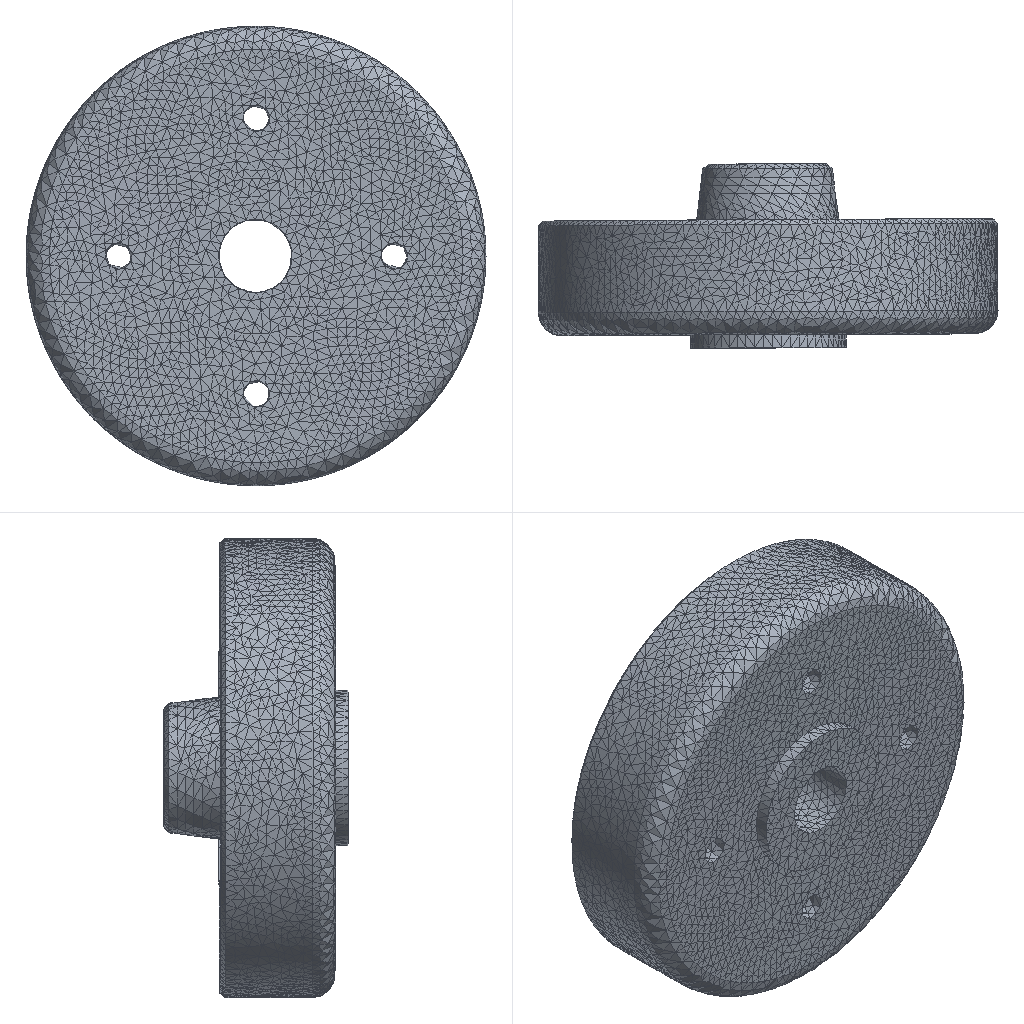Simulation study | ansys workbench
Set-up summary:
category,name,step,type,value,unit,region
solver,ansys_workbench
units,mm-N-s-tonne (MPa),,stated,"/units,MPA"
analysis,LS1,,modal,method=lanb; n_modes=6
load_step,LS1,LS1,modal
mesh,nodes,,,55175
mesh,elements,,,31822
element_type,SOLID187,,,31822
material,Gray Cast Iron,,E,110000,tonne s^-2 mm^-1
material,Gray Cast Iron,,nu,0.28
material,Gray Cast Iron,,density,7.2e-09,tonne mm^-3
material,Gray Cast Iron,,conductivity,52,tonne mm s^-3 C^-1
material,Gray Cast Iron,,specific_heat,4.47e+08,mm^2 s^-2 C^-1
material,Gray Cast Iron,,cte,1.1e-05,C^-1
material,Gray Cast Iron,,permeability,10000
material,Gray Cast Iron,,resistivity,9.6e-05,ohm mm
bc,Fixed Supports,model,fixed,[dofs=ALL],,_FIXEDSU
named_set,_FIXEDSU,,node,820
Ansys APDL input file, long lists of numbers shortened:
/batch
/config,noeldb,1     ! force off writing results to database
*get,_wallstrt,active,,time,wall
! ANSYS input file written by Workbench version 2022 R2
! File used for geometry attach:
/title,wbnew--__ (A5)
! ****** Begin Custom Load Command Snippet ******
/COM, ACT Extensions:
/COM,     LSDYNA, 2022.2
/COM,/COM,     ANSYSMotion, 2022.2
/COM,
! ****** End   Custom Load Command Snippet ******
*DIM,_wb_ProjectScratch_dir,string,248
_wb_ProjectScratch_dir(1) = ''
*DIM,_wb_SolverFiles_dir,string,248
_wb_SolverFiles_dir(1) = ''
*DIM,_wb_userfiles_dir,string,248
_wb_userfiles_dir(1) = ''
/com,--- Data in consistent NMM units. See Solving Units in the help system for more information.
/units,MPA
/nopr
/wb,file,start              !  signify a WB generated input file
/prep7
! Turn off shape checking because checks already performed inside WB mesher.
! See help system for more information.
SHPP,OFF,,NOWARN
/nolist
etcon,set             ! allow ANSYS to choose best KEYOP's for 180x elements, resets any applicable keyopt to MAPDL defaults
/com,*********** Nodes for the whole assembly ***********
nblock,3,,60692
(1i9,3e20.9e3)
        1    -4.498793260E+01     2.959381846E+00    -5.507709401E-15
! (55174 more lines like these left out)
-1
/wb,elem,start            !  set before creation of elements
/com,*********** Elements for Body 1 "Part 1" ***********
et,1,187
eblock,19,solid,,31822
(19i9)
        1        1        1        1        0        0        0        0       10        0        1     2717     2878     8600     6506    24930    25799    24933    24932
! (63643 more lines like these left out)
-1
/wb,elem,end               !  done creating elements
/com,*********** Send User Defined Coordinate System(s) ***********
csys,0
toffst,273.15,  ! Temperature offset from absolute zero
/com,*********** Set Reference Temperature ***********
tref,22.
/wb,mat,start              !  starting to send materials
/com,*********** Send Materials ***********
Temperature = 'TEMP' ! Temperature
MP,DENS,1,7.2e-09,	! tonne mm^-3
MP,ALPX,1,1.1e-05,	! C^-1
MP,C,1,447000000,	! mm^2 s^-2 C^-1
MP,KXX,1,52,	! tonne mm s^-3 C^-1
MP,RSVX,1,9.6e-05,	! ohm mm
MP,EX,1,110000,	! tonne s^-2 mm^-1
MP,NUXY,1,0.28,
MP,MURX,1,10000,
/wb,mat,end                !  done sending materials
!************************* Model Summary ********************
!Part 1,	灰铸铁,	matid,	1
!************************* End Model Summary ********************
! get the diagonal of the bounding box. Needed later for other things
*get,_xmin,node,,mnloc,x
*get,_ymin,node,,mnloc,y
*get,_zmin,node,,mnloc,z
*get,_xmax,node,,mxloc,x
*get,_ymax,node,,mxloc,y
*get,_zmax,node,,mxloc,z
_ASMDIAG=(_xmax-_xmin)*(_xmax-_xmin)+(_ymax-_ymin)*(_ymax-_ymin)+(_zmax-_zmin)*(_zmax-_zmin)
_ASMDIAG=SQRT(_ASMDIAG)
/wb,contact,start          !  starting to send contact
/wb,contact,end            !  done creating contacts
/golist
/wb,load,start             !  starting to send loads
/com,*********** Fixed Supports ***********
CMBLOCK,_FIXEDSU,NODE,      820
(8i10)
       197       198       199       200       201       202       203       204
! (102 more lines like these left out)
cmsel,s,_FIXEDSU
d,all,all
nsel,all
/gst,on,on
fini
*get,_numnode,node,0,count
*get,_numelem,elem,0,count
*get, _MAXELEMNUM, elem, 0, NUM, MAX
*get, _MAXNODENUM, node, 0, NUM, MAX
*get, _MAXELEMTYPE, etyp, 0, NUM, MAX
*get, _MAXREALCONST, rcon, 0, NUM, MAX
/go
/wb,load,end               !  done creating loads
/com,--- Number of total nodes = %_numnode%
/com,--- Number of contact elements = 0
/com,--- Number of spring elements = 0
/com,--- Number of bearing elements = 0
/com,--- Number of solid elements = 31822
/com,--- Number of condensed parts = 0
/com,--- Number of total elements = %_numelem%
*get,_wallbsol,active,,time,wall
/solu
antype,2                   ! modal analysis
_thickRatio=  1     ! Ratio of thick parts in the model
modopt,lanb,6
outres,erase
outres,all,none
outres,nsol,all
mxpand                    ! default expand in case of complex solution
dmpopt,esav,no
dmpopt,emat,no
dmpopt,full,no
! *********** WB SOLVE COMMAND ***********
! check interactive state
*get,ANSINTER_,active,,int
*if,ANSINTER_,ne,0,then
/eof
*endif
solve
/com *************** Write FE CONNECTORS *********
CEWRITE,file,ce,,INTE
*get,_nmodalsolproc,active,0,numcpu
fini
/nopr
*get,_numnode,node,0,count
*get,_numelem,elem,0,count
*get, _MAXELEMNUM, elem, 0, NUM, MAX
*get, _MAXNODENUM, node, 0, NUM, MAX,,,INTERNAL
*get, _MAXELEMTYPE, etyp, 0, NUM, MAX
*get, _MAXREALCONST, rcon, 0, NUM, MAX
*get,_NSOLTHREADS,active,0,ntfs
*get,_NSOLPROCESSES,active,0,npfs
/gopr
*get,_wallasol,active,,time,wall
/post1
/nopr
*dim,_direction,CHAR,6,1
_direction(1) = 'X'
_direction(2) = 'Y'
_direction(3) = 'Z'
_direction(4) = 'ROTX'
_direction(5) = 'ROTY'
_direction(6) = 'ROTZ'
*get,_lastLS,active,0,set,LSTP
*get,_beginset,active,0,set,nset,first,_lastLS
*get,_endset,active,0,set,nset,last,_lastLS
_nummodes = 0
*if,_endset,gt,0,then
_nummodes = _endset - _beginset + 1
*endif
*do,i_mode,1,_nummodes
   *do,j_component,1,6
			*get,PFACT_%i_mode%_%j_component%,MODE,%i_mode%,PFACT,,DIREC,_direction(%j_component%)
   *enddo
*enddo
*dim,_tmdirection,CHAR,6,1
_tmdirection(1) = 'X'
_tmdirection(2) = 'Y'
_tmdirection(3) = 'Z'
_tmdirection(4) = 'X'
_tmdirection(5) = 'Y'
_tmdirection(6) = 'Z'
*do,j_component,1,6
    *if,j_component,gt,3,then
        *get,TOTALMASS_%j_component%,ELEM,0,IOR,_tmdirection(%j_component%)
    *else
        *get,TOTALMASS_%j_component%,ELEM,0,MTOT,_tmdirection(%j_component%)
    *endif
*enddo
/gopr
xmlo,ENCODING,ISO-8859-1
xmlo,parm
/xml,parm,xml
fini
/gopr
*get,_walldone,active,,time,wall
_preptime=(_wallbsol-_wallstrt)*3600
_solvtime=(_wallasol-_wallbsol)*3600
_posttime=(_walldone-_wallasol)*3600
_totaltim=(_walldone-_wallstrt)*3600
*get,_dlbratio,active,0,solu,dlbr
*get,_combtime,active,0,solu,comb
*get,_ssmode,active,0,solu,ssmm
*get,_ndofs,active,0,solu,ndof
/fclean				!clean distributed files
/com,--- Total number of nodes = %_numnode%
/com,--- Total number of elements = %_numelem%
/com,--- Element load balance ratio = %_dlbratio%
/com,--- Time to combine distributed files = %_combtime%
/com,--- Sparse memory mode = %_ssmode%
/com,--- Number of DOF = %_ndofs%
/wb,file,end               ! done with WB generated input
Results summary:
result,analyses[0].index,,,1
result,analyses[0].system,,,SYS
result,analyses[0].deck,,,deck.dat
result,analyses[0].solve_status,,,completed
result,analyses[0].analysis_type,,,modal
result,analyses[0].physics,,,mechanical
result,analyses[0].unit_system,,,"NMM: mm, ton, N, s, mV, mA, degC"
result,analyses[0].n_sets,,,6
result,analyses[0].modal_frequencies_hz[1],,,6761.81
result,analyses[0].modal_frequencies_hz[2],,,7752.92
result,analyses[0].modal_frequencies_hz[3],,,7754.68
result,analyses[0].modal_frequencies_hz[4],,,8945.07
result,analyses[0].modal_frequencies_hz[5],,,9941.12
result,analyses[0].modal_frequencies_hz[6],,,11813.9